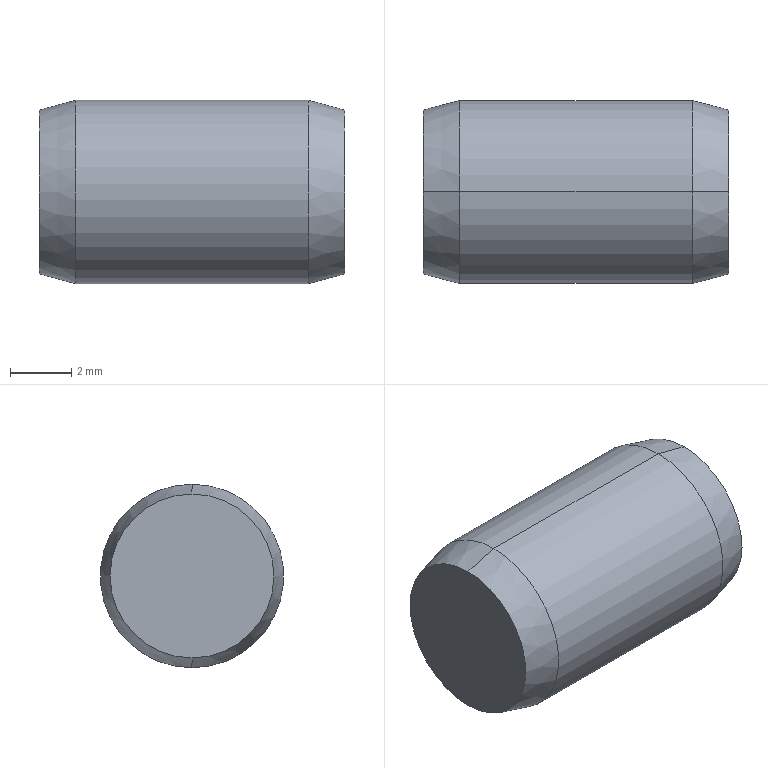Part | SolidWorks | features BaseBody 1 | 1 solid | 8 faces | box 10 x 6 x 6 mm | volume 275.73 mm3 | cone 4 | cylinder 2 | plane 2 | commonest cylinder face diameters 6 x2
STEP:
#1=CARTESIAN_POINT('',(-5.,0.,2.678));
#2=VERTEX_POINT('',#1);
#3=CARTESIAN_POINT('',(-5.,0.,-2.678));
#4=VERTEX_POINT('',#3);
#5=CARTESIAN_POINT('',(-5.,0.,0.));
#6=DIRECTION('',(-1.,0.,0.));
#7=DIRECTION('',(0.,0.,1.));
#8=AXIS2_PLACEMENT_3D('',#5,#6,#7);
#9=CIRCLE('',#8,2.678);
#10=EDGE_CURVE('',#2,#4,#9,.T.);
#11=ORIENTED_EDGE('',*,*,#10,.F.);
#12=CARTESIAN_POINT('',(-3.8,0.,3.));
#13=VERTEX_POINT('',#12);
#14=CARTESIAN_POINT('',(-3.8,0.,3.));
#15=DIRECTION('',(0.9659,0.,0.2588));
#16=VECTOR('',#15,1000.);
#17=LINE('',#14,#16);
#18=EDGE_CURVE('',#2,#13,#17,.T.);
#19=ORIENTED_EDGE('',*,*,#18,.T.);
#20=CARTESIAN_POINT('',(-3.8,0.,-3.));
#21=VERTEX_POINT('',#20);
#22=CARTESIAN_POINT('',(-3.8,0.,0.));
#23=DIRECTION('',(-1.,0.,0.));
#24=DIRECTION('',(0.,0.,1.));
#25=AXIS2_PLACEMENT_3D('',#22,#23,#24);
#26=CIRCLE('',#25,3.);
#27=EDGE_CURVE('',#13,#21,#26,.T.);
#28=ORIENTED_EDGE('',*,*,#27,.T.);
#29=CARTESIAN_POINT('',(-3.8,0.,-3.));
#30=DIRECTION('',(0.9659,0.,-0.2588));
#31=VECTOR('',#30,1000.);
#32=LINE('',#29,#31);
#33=EDGE_CURVE('',#4,#21,#32,.T.);
#34=ORIENTED_EDGE('',*,*,#33,.F.);
#35=EDGE_LOOP('',(#11,#19,#28,#34));
#36=FACE_OUTER_BOUND('',#35,.T.);
#37=CARTESIAN_POINT('',(-3.8,0.,0.));
#38=DIRECTION('',(1.,0.,0.));
#39=DIRECTION('',(0.,0.,-1.));
#40=AXIS2_PLACEMENT_3D('',#37,#38,#39);
#41=CONICAL_SURFACE('',#40,3.,0.2618);
#42=ADVANCED_FACE('',(#36),#41,.T.);
#43=CARTESIAN_POINT('',(3.8,0.,3.));
#44=VERTEX_POINT('',#43);
#45=CARTESIAN_POINT('',(3.8,0.,-3.));
#46=VERTEX_POINT('',#45);
#47=CARTESIAN_POINT('',(3.8,0.,0.));
#48=DIRECTION('',(-1.,0.,0.));
#49=DIRECTION('',(0.,0.,1.));
#50=AXIS2_PLACEMENT_3D('',#47,#48,#49);
#51=CIRCLE('',#50,3.);
#52=EDGE_CURVE('',#44,#46,#51,.T.);
#53=ORIENTED_EDGE('',*,*,#52,.T.);
#54=CARTESIAN_POINT('',(-5.,0.,-3.));
#55=DIRECTION('',(-1.,0.,0.));
#56=VECTOR('',#55,1000.);
#57=LINE('',#54,#56);
#58=EDGE_CURVE('',#46,#21,#57,.T.);
#59=ORIENTED_EDGE('',*,*,#58,.T.);
#60=ORIENTED_EDGE('',*,*,#27,.F.);
#61=CARTESIAN_POINT('',(-5.,0.,3.));
#62=DIRECTION('',(-1.,0.,0.));
#63=VECTOR('',#62,1000.);
#64=LINE('',#61,#63);
#65=EDGE_CURVE('',#44,#13,#64,.T.);
#66=ORIENTED_EDGE('',*,*,#65,.F.);
#67=EDGE_LOOP('',(#53,#59,#60,#66));
#68=FACE_OUTER_BOUND('',#67,.T.);
#69=CARTESIAN_POINT('',(-5.,0.,0.));
#70=DIRECTION('',(-1.,0.,0.));
#71=DIRECTION('',(0.,0.,1.));
#72=AXIS2_PLACEMENT_3D('',#69,#70,#71);
#73=CYLINDRICAL_SURFACE('',#72,3.);
#74=ADVANCED_FACE('',(#68),#73,.T.);
#75=CARTESIAN_POINT('',(5.,0.,2.678));
#76=VERTEX_POINT('',#75);
#77=CARTESIAN_POINT('',(5.,0.,-2.678));
#78=VERTEX_POINT('',#77);
#79=CARTESIAN_POINT('',(5.,0.,0.));
#80=DIRECTION('',(-1.,0.,0.));
#81=DIRECTION('',(0.,0.,1.));
#82=AXIS2_PLACEMENT_3D('',#79,#80,#81);
#83=CIRCLE('',#82,2.678);
#84=EDGE_CURVE('',#76,#78,#83,.T.);
#85=ORIENTED_EDGE('',*,*,#84,.T.);
#86=CARTESIAN_POINT('',(5.,0.,-2.678));
#87=DIRECTION('',(-0.9659,0.,-0.2588));
#88=VECTOR('',#87,1000.);
#89=LINE('',#86,#88);
#90=EDGE_CURVE('',#78,#46,#89,.T.);
#91=ORIENTED_EDGE('',*,*,#90,.T.);
#92=ORIENTED_EDGE('',*,*,#52,.F.);
#93=CARTESIAN_POINT('',(5.,0.,2.678));
#94=DIRECTION('',(-0.9659,0.,0.2588));
#95=VECTOR('',#94,1000.);
#96=LINE('',#93,#95);
#97=EDGE_CURVE('',#76,#44,#96,.T.);
#98=ORIENTED_EDGE('',*,*,#97,.F.);
#99=EDGE_LOOP('',(#85,#91,#92,#98));
#100=FACE_OUTER_BOUND('',#99,.T.);
#101=CARTESIAN_POINT('',(5.,0.,0.));
#102=DIRECTION('',(-1.,0.,0.));
#103=DIRECTION('',(0.,0.,1.));
#104=AXIS2_PLACEMENT_3D('',#101,#102,#103);
#105=CONICAL_SURFACE('',#104,2.678,0.2618);
#106=ADVANCED_FACE('',(#100),#105,.T.);
#107=ORIENTED_EDGE('',*,*,#84,.F.);
#108=CARTESIAN_POINT('',(5.,0.,0.));
#109=DIRECTION('',(-1.,0.,0.));
#110=DIRECTION('',(0.,0.,1.));
#111=AXIS2_PLACEMENT_3D('',#108,#109,#110);
#112=CIRCLE('',#111,2.678);
#113=EDGE_CURVE('',#78,#76,#112,.T.);
#114=ORIENTED_EDGE('',*,*,#113,.F.);
#115=EDGE_LOOP('',(#107,#114));
#116=FACE_OUTER_BOUND('',#115,.T.);
#117=CARTESIAN_POINT('',(5.,0.,0.));
#118=DIRECTION('',(-1.,0.,0.));
#119=DIRECTION('',(0.,0.,1.));
#120=AXIS2_PLACEMENT_3D('',#117,#118,#119);
#121=PLANE('',#120);
#122=ADVANCED_FACE('',(#116),#121,.F.);
#123=CARTESIAN_POINT('',(-5.,0.,0.));
#124=DIRECTION('',(-1.,0.,0.));
#125=DIRECTION('',(0.,0.,1.));
#126=AXIS2_PLACEMENT_3D('',#123,#124,#125);
#127=CIRCLE('',#126,2.678);
#128=EDGE_CURVE('',#4,#2,#127,.T.);
#129=ORIENTED_EDGE('',*,*,#128,.T.);
#130=ORIENTED_EDGE('',*,*,#10,.T.);
#131=EDGE_LOOP('',(#129,#130));
#132=FACE_OUTER_BOUND('',#131,.T.);
#133=CARTESIAN_POINT('',(-5.,2.678,0.));
#134=DIRECTION('',(1.,0.,0.));
#135=DIRECTION('',(0.,1.,0.));
#136=AXIS2_PLACEMENT_3D('',#133,#134,#135);
#137=PLANE('',#136);
#138=ADVANCED_FACE('',(#132),#137,.F.);
#139=ORIENTED_EDGE('',*,*,#90,.F.);
#140=ORIENTED_EDGE('',*,*,#113,.T.);
#141=ORIENTED_EDGE('',*,*,#97,.T.);
#142=CARTESIAN_POINT('',(3.8,0.,0.));
#143=DIRECTION('',(-1.,0.,0.));
#144=DIRECTION('',(0.,0.,1.));
#145=AXIS2_PLACEMENT_3D('',#142,#143,#144);
#146=CIRCLE('',#145,3.);
#147=EDGE_CURVE('',#46,#44,#146,.T.);
#148=ORIENTED_EDGE('',*,*,#147,.F.);
#149=EDGE_LOOP('',(#139,#140,#141,#148));
#150=FACE_OUTER_BOUND('',#149,.T.);
#151=CARTESIAN_POINT('',(5.,0.,0.));
#152=DIRECTION('',(-1.,0.,0.));
#153=DIRECTION('',(0.,0.,1.));
#154=AXIS2_PLACEMENT_3D('',#151,#152,#153);
#155=CONICAL_SURFACE('',#154,2.678,0.2618);
#156=ADVANCED_FACE('',(#150),#155,.T.);
#157=ORIENTED_EDGE('',*,*,#58,.F.);
#158=ORIENTED_EDGE('',*,*,#147,.T.);
#159=ORIENTED_EDGE('',*,*,#65,.T.);
#160=CARTESIAN_POINT('',(-3.8,0.,0.));
#161=DIRECTION('',(-1.,0.,0.));
#162=DIRECTION('',(0.,0.,1.));
#163=AXIS2_PLACEMENT_3D('',#160,#161,#162);
#164=CIRCLE('',#163,3.);
#165=EDGE_CURVE('',#21,#13,#164,.T.);
#166=ORIENTED_EDGE('',*,*,#165,.F.);
#167=EDGE_LOOP('',(#157,#158,#159,#166));
#168=FACE_OUTER_BOUND('',#167,.T.);
#169=CARTESIAN_POINT('',(-5.,0.,0.));
#170=DIRECTION('',(-1.,0.,0.));
#171=DIRECTION('',(0.,0.,1.));
#172=AXIS2_PLACEMENT_3D('',#169,#170,#171);
#173=CYLINDRICAL_SURFACE('',#172,3.);
#174=ADVANCED_FACE('',(#168),#173,.T.);
#175=ORIENTED_EDGE('',*,*,#18,.F.);
#176=ORIENTED_EDGE('',*,*,#128,.F.);
#177=ORIENTED_EDGE('',*,*,#33,.T.);
#178=ORIENTED_EDGE('',*,*,#165,.T.);
#179=EDGE_LOOP('',(#175,#176,#177,#178));
#180=FACE_OUTER_BOUND('',#179,.T.);
#181=CARTESIAN_POINT('',(-3.8,0.,0.));
#182=DIRECTION('',(1.,0.,0.));
#183=DIRECTION('',(0.,0.,-1.));
#184=AXIS2_PLACEMENT_3D('',#181,#182,#183);
#185=CONICAL_SURFACE('',#184,3.,0.2618);
#186=ADVANCED_FACE('',(#180),#185,.T.);
#187=CLOSED_SHELL('',(#42,#74,#106,#122,#138,#156,#174,#186));
#188=MANIFOLD_SOLID_BREP('',#187);
#189=CARTESIAN_POINT('',(0.,0.,0.));
#190=DIRECTION('',(0.,0.,1.));
#191=DIRECTION('',(1.,0.,0.));
#192=AXIS2_PLACEMENT_3D('',#189,#190,#191);
#193=(LENGTH_UNIT()NAMED_UNIT(*)SI_UNIT(.MILLI.,.METRE.));
#194=UNCERTAINTY_MEASURE_WITH_UNIT(LENGTH_MEASURE(0.00001),#193,'','');
#195=(NAMED_UNIT(*)PLANE_ANGLE_UNIT()SI_UNIT($,.RADIAN.));
#196=(NAMED_UNIT(*)SI_UNIT($,.STERADIAN.)SOLID_ANGLE_UNIT());
#197=(GEOMETRIC_REPRESENTATION_CONTEXT(3)GLOBAL_UNCERTAINTY_ASSIGNED_CONTEXT((#194))GLOBAL_UNIT_ASSIGNED_CONTEXT((#193,#195,#196))REPRESENTATION_CONTEXT('',''));
#198=ADVANCED_BREP_SHAPE_REPRESENTATION('',(#188,#192),#197);